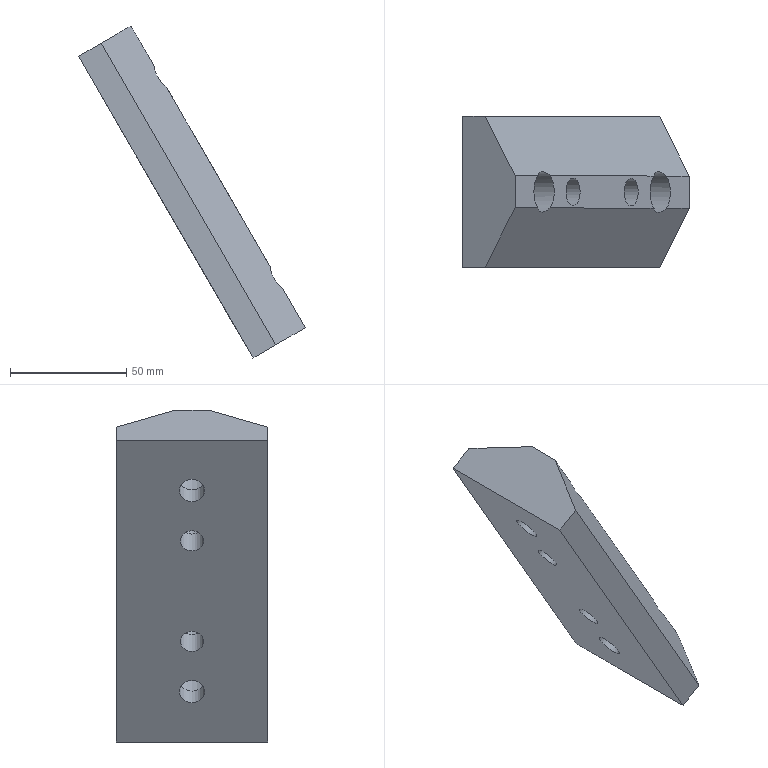Part | NX | features solid 2 | 1 solid | 22 faces | box 97.517 x 65 x 142.904 mm | volume 182430 mm3 | plane 12 | cylinder 8 | cone 2 | commonest cylinder face diameters 10 x2 11 x2 12 x2 17.5 x2
STEP:
#1=CARTESIAN_POINT('',(-987.747,-43.072,-36.314));
#2=VERTEX_POINT('',#1);
#3=CARTESIAN_POINT('',(-977.919,-43.072,-53.336));
#4=VERTEX_POINT('',#3);
#5=CARTESIAN_POINT('',(-1052.919,-43.072,76.567));
#6=DIRECTION('',(0.5,0.,-0.866));
#7=VECTOR('',#6,1000.);
#8=LINE('',#5,#7);
#9=EDGE_CURVE('',#2,#4,#8,.T.);
#10=ORIENTED_EDGE('',*,*,#9,.F.);
#11=CARTESIAN_POINT('',(-987.747,-56.928,-36.314));
#12=VERTEX_POINT('',#11);
#13=CARTESIAN_POINT('',(-990.419,-50.,-31.686));
#14=DIRECTION('',(0.866,0.,0.5));
#15=DIRECTION('',(0.5,0.,-0.866));
#16=AXIS2_PLACEMENT_3D('',#13,#14,#15);
#17=CIRCLE('',#16,8.75);
#18=EDGE_CURVE('',#12,#2,#17,.T.);
#19=ORIENTED_EDGE('',*,*,#18,.F.);
#20=CARTESIAN_POINT('',(-977.919,-56.928,-53.336));
#21=VERTEX_POINT('',#20);
#22=CARTESIAN_POINT('',(-1052.919,-56.928,76.567));
#23=DIRECTION('',(0.5,0.,-0.866));
#24=VECTOR('',#23,1000.);
#25=LINE('',#22,#24);
#26=EDGE_CURVE('',#12,#21,#25,.T.);
#27=ORIENTED_EDGE('',*,*,#26,.T.);
#28=CARTESIAN_POINT('',(-977.919,-17.5,-53.336));
#29=DIRECTION('',(0.,-1.,0.));
#30=VECTOR('',#29,1000.);
#31=LINE('',#28,#30);
#32=EDGE_CURVE('',#4,#21,#31,.T.);
#33=ORIENTED_EDGE('',*,*,#32,.F.);
#34=EDGE_LOOP('',(#10,#19,#27,#33));
#35=FACE_BOUND('',#34,.T.);
#36=CARTESIAN_POINT('',(-977.919,-17.5,-53.336));
#37=DIRECTION('',(-0.866,0.,-0.5));
#38=DIRECTION('',(0.5,0.,-0.866));
#39=AXIS2_PLACEMENT_3D('',#36,#37,#38);
#40=PLANE('',#39);
#41=ADVANCED_FACE('',(#35),#40,.F.);
#42=CARTESIAN_POINT('',(-1037.747,-43.072,50.288));
#43=VERTEX_POINT('',#42);
#44=CARTESIAN_POINT('',(-993.092,-43.072,-27.057));
#45=VERTEX_POINT('',#44);
#46=CARTESIAN_POINT('',(-1052.919,-43.072,76.567));
#47=DIRECTION('',(0.5,0.,-0.866));
#48=VECTOR('',#47,1000.);
#49=LINE('',#46,#48);
#50=EDGE_CURVE('',#43,#45,#49,.T.);
#51=ORIENTED_EDGE('',*,*,#50,.F.);
#52=CARTESIAN_POINT('',(-1037.747,-56.928,50.288));
#53=VERTEX_POINT('',#52);
#54=CARTESIAN_POINT('',(-1040.419,-50.,54.917));
#55=DIRECTION('',(0.866,0.,0.5));
#56=DIRECTION('',(0.5,0.,-0.866));
#57=AXIS2_PLACEMENT_3D('',#54,#55,#56);
#58=CIRCLE('',#57,8.75);
#59=EDGE_CURVE('',#53,#43,#58,.T.);
#60=ORIENTED_EDGE('',*,*,#59,.F.);
#61=CARTESIAN_POINT('',(-993.092,-56.928,-27.057));
#62=VERTEX_POINT('',#61);
#63=CARTESIAN_POINT('',(-1052.919,-56.928,76.567));
#64=DIRECTION('',(0.5,0.,-0.866));
#65=VECTOR('',#64,1000.);
#66=LINE('',#63,#65);
#67=EDGE_CURVE('',#53,#62,#66,.T.);
#68=ORIENTED_EDGE('',*,*,#67,.T.);
#69=CARTESIAN_POINT('',(-990.419,-50.,-31.686));
#70=DIRECTION('',(0.866,0.,0.5));
#71=DIRECTION('',(0.5,0.,-0.866));
#72=AXIS2_PLACEMENT_3D('',#69,#70,#71);
#73=CIRCLE('',#72,8.75);
#74=EDGE_CURVE('',#45,#62,#73,.T.);
#75=ORIENTED_EDGE('',*,*,#74,.F.);
#76=EDGE_LOOP('',(#51,#60,#68,#75));
#77=FACE_BOUND('',#76,.T.);
#78=CARTESIAN_POINT('',(-999.919,-50.,-15.231));
#79=VERTEX_POINT('',#78);
#80=CARTESIAN_POINT('',(-1002.919,-50.,-10.035));
#81=DIRECTION('',(0.866,0.,0.5));
#82=DIRECTION('',(0.5,0.,-0.866));
#83=AXIS2_PLACEMENT_3D('',#80,#81,#82);
#84=CIRCLE('',#83,6.);
#85=EDGE_CURVE('',#79,#79,#84,.T.);
#86=ORIENTED_EDGE('',*,*,#85,.F.);
#87=EDGE_LOOP('',(#86));
#88=FACE_BOUND('',#87,.T.);
#89=CARTESIAN_POINT('',(-1024.919,-50.,28.07));
#90=VERTEX_POINT('',#89);
#91=CARTESIAN_POINT('',(-1027.919,-50.,33.266));
#92=DIRECTION('',(0.866,0.,0.5));
#93=DIRECTION('',(0.5,0.,-0.866));
#94=AXIS2_PLACEMENT_3D('',#91,#92,#93);
#95=CIRCLE('',#94,6.);
#96=EDGE_CURVE('',#90,#90,#95,.T.);
#97=ORIENTED_EDGE('',*,*,#96,.F.);
#98=EDGE_LOOP('',(#97));
#99=FACE_BOUND('',#98,.T.);
#100=CARTESIAN_POINT('',(-977.919,-17.5,-53.336));
#101=DIRECTION('',(-0.866,0.,-0.5));
#102=DIRECTION('',(0.5,0.,-0.866));
#103=AXIS2_PLACEMENT_3D('',#100,#101,#102);
#104=PLANE('',#103);
#105=ADVANCED_FACE('',(#77,#88,#99),#104,.F.);
#106=CARTESIAN_POINT('',(-990.705,-17.5,-60.718));
#107=VERTEX_POINT('',#106);
#108=CARTESIAN_POINT('',(-977.919,-43.072,-53.336));
#109=DIRECTION('',(-0.433,0.866,-0.25));
#110=VECTOR('',#109,1000.);
#111=LINE('',#108,#110);
#112=EDGE_CURVE('',#4,#107,#111,.T.);
#113=ORIENTED_EDGE('',*,*,#112,.F.);
#114=ORIENTED_EDGE('',*,*,#32,.T.);
#115=CARTESIAN_POINT('',(-990.705,-82.5,-60.718));
#116=VERTEX_POINT('',#115);
#117=CARTESIAN_POINT('',(-990.705,-82.5,-60.718));
#118=DIRECTION('',(0.433,0.866,0.25));
#119=VECTOR('',#118,1000.);
#120=LINE('',#117,#119);
#121=EDGE_CURVE('',#116,#21,#120,.T.);
#122=ORIENTED_EDGE('',*,*,#121,.F.);
#123=CARTESIAN_POINT('',(-1000.436,-82.5,-66.336));
#124=VERTEX_POINT('',#123);
#125=CARTESIAN_POINT('',(-977.919,-82.5,-53.336));
#126=DIRECTION('',(-0.866,0.,-0.5));
#127=VECTOR('',#126,1000.);
#128=LINE('',#125,#127);
#129=EDGE_CURVE('',#116,#124,#128,.T.);
#130=ORIENTED_EDGE('',*,*,#129,.T.);
#131=CARTESIAN_POINT('',(-1000.436,-17.5,-66.336));
#132=VERTEX_POINT('',#131);
#133=CARTESIAN_POINT('',(-1000.436,-17.5,-66.336));
#134=DIRECTION('',(0.,-1.,0.));
#135=VECTOR('',#134,1000.);
#136=LINE('',#133,#135);
#137=EDGE_CURVE('',#132,#124,#136,.T.);
#138=ORIENTED_EDGE('',*,*,#137,.F.);
#139=CARTESIAN_POINT('',(-977.919,-17.5,-53.336));
#140=DIRECTION('',(-0.866,0.,-0.5));
#141=VECTOR('',#140,1000.);
#142=LINE('',#139,#141);
#143=EDGE_CURVE('',#107,#132,#142,.T.);
#144=ORIENTED_EDGE('',*,*,#143,.F.);
#145=EDGE_LOOP('',(#113,#114,#122,#130,#138,#144));
#146=FACE_BOUND('',#145,.T.);
#147=CARTESIAN_POINT('',(-977.919,-17.5,-53.336));
#148=DIRECTION('',(-0.5,0.,0.866));
#149=DIRECTION('',(0.,1.,0.));
#150=AXIS2_PLACEMENT_3D('',#147,#148,#149);
#151=PLANE('',#150);
#152=ADVANCED_FACE('',(#146),#151,.F.);
#153=CARTESIAN_POINT('',(-1065.705,-82.5,69.185));
#154=VERTEX_POINT('',#153);
#155=CARTESIAN_POINT('',(-1065.705,-82.5,69.185));
#156=DIRECTION('',(0.5,0.,-0.866));
#157=VECTOR('',#156,1000.);
#158=LINE('',#155,#157);
#159=EDGE_CURVE('',#154,#116,#158,.T.);
#160=ORIENTED_EDGE('',*,*,#159,.F.);
#161=CARTESIAN_POINT('',(-1075.436,-82.5,63.567));
#162=VERTEX_POINT('',#161);
#163=CARTESIAN_POINT('',(-1052.919,-82.5,76.567));
#164=DIRECTION('',(-0.866,0.,-0.5));
#165=VECTOR('',#164,1000.);
#166=LINE('',#163,#165);
#167=EDGE_CURVE('',#154,#162,#166,.T.);
#168=ORIENTED_EDGE('',*,*,#167,.T.);
#169=CARTESIAN_POINT('',(-1000.436,-82.5,-66.336));
#170=DIRECTION('',(-0.5,0.,0.866));
#171=VECTOR('',#170,1000.);
#172=LINE('',#169,#171);
#173=EDGE_CURVE('',#124,#162,#172,.T.);
#174=ORIENTED_EDGE('',*,*,#173,.F.);
#175=ORIENTED_EDGE('',*,*,#129,.F.);
#176=EDGE_LOOP('',(#160,#168,#174,#175));
#177=FACE_BOUND('',#176,.T.);
#178=CARTESIAN_POINT('',(-977.919,-82.5,-53.336));
#179=DIRECTION('',(0.,1.,0.));
#180=DIRECTION('',(0.5,0.,-0.866));
#181=AXIS2_PLACEMENT_3D('',#178,#179,#180);
#182=PLANE('',#181);
#183=ADVANCED_FACE('',(#177),#182,.F.);
#184=CARTESIAN_POINT('',(-1052.919,-43.072,76.567));
#185=VERTEX_POINT('',#184);
#186=CARTESIAN_POINT('',(-1065.705,-17.5,69.185));
#187=VERTEX_POINT('',#186);
#188=CARTESIAN_POINT('',(-1052.919,-43.072,76.567));
#189=DIRECTION('',(-0.433,0.866,-0.25));
#190=VECTOR('',#189,1000.);
#191=LINE('',#188,#190);
#192=EDGE_CURVE('',#185,#187,#191,.T.);
#193=ORIENTED_EDGE('',*,*,#192,.T.);
#194=CARTESIAN_POINT('',(-1075.436,-17.5,63.567));
#195=VERTEX_POINT('',#194);
#196=CARTESIAN_POINT('',(-1052.919,-17.5,76.567));
#197=DIRECTION('',(-0.866,0.,-0.5));
#198=VECTOR('',#197,1000.);
#199=LINE('',#196,#198);
#200=EDGE_CURVE('',#187,#195,#199,.T.);
#201=ORIENTED_EDGE('',*,*,#200,.T.);
#202=CARTESIAN_POINT('',(-1075.436,-82.5,63.567));
#203=DIRECTION('',(0.,1.,0.));
#204=VECTOR('',#203,1000.);
#205=LINE('',#202,#204);
#206=EDGE_CURVE('',#162,#195,#205,.T.);
#207=ORIENTED_EDGE('',*,*,#206,.F.);
#208=ORIENTED_EDGE('',*,*,#167,.F.);
#209=CARTESIAN_POINT('',(-1052.919,-56.928,76.567));
#210=VERTEX_POINT('',#209);
#211=CARTESIAN_POINT('',(-1065.705,-82.5,69.185));
#212=DIRECTION('',(0.433,0.866,0.25));
#213=VECTOR('',#212,1000.);
#214=LINE('',#211,#213);
#215=EDGE_CURVE('',#154,#210,#214,.T.);
#216=ORIENTED_EDGE('',*,*,#215,.T.);
#217=CARTESIAN_POINT('',(-1052.919,-82.5,76.567));
#218=DIRECTION('',(0.,1.,0.));
#219=VECTOR('',#218,1000.);
#220=LINE('',#217,#219);
#221=EDGE_CURVE('',#210,#185,#220,.T.);
#222=ORIENTED_EDGE('',*,*,#221,.T.);
#223=EDGE_LOOP('',(#193,#201,#207,#208,#216,#222));
#224=FACE_BOUND('',#223,.T.);
#225=CARTESIAN_POINT('',(-1052.919,-82.5,76.567));
#226=DIRECTION('',(0.5,0.,-0.866));
#227=DIRECTION('',(0.866,0.,0.5));
#228=AXIS2_PLACEMENT_3D('',#225,#226,#227);
#229=PLANE('',#228);
#230=ADVANCED_FACE('',(#224),#229,.F.);
#231=CARTESIAN_POINT('',(-1065.705,-17.5,69.185));
#232=DIRECTION('',(0.5,0.,-0.866));
#233=VECTOR('',#232,1000.);
#234=LINE('',#231,#233);
#235=EDGE_CURVE('',#187,#107,#234,.T.);
#236=ORIENTED_EDGE('',*,*,#235,.T.);
#237=ORIENTED_EDGE('',*,*,#143,.T.);
#238=CARTESIAN_POINT('',(-1075.436,-17.5,63.567));
#239=DIRECTION('',(0.5,0.,-0.866));
#240=VECTOR('',#239,1000.);
#241=LINE('',#238,#240);
#242=EDGE_CURVE('',#195,#132,#241,.T.);
#243=ORIENTED_EDGE('',*,*,#242,.F.);
#244=ORIENTED_EDGE('',*,*,#200,.F.);
#245=EDGE_LOOP('',(#236,#237,#243,#244));
#246=FACE_BOUND('',#245,.T.);
#247=CARTESIAN_POINT('',(-1052.919,-17.5,76.567));
#248=DIRECTION('',(0.,-1.,0.));
#249=DIRECTION('',(-0.5,0.,0.866));
#250=AXIS2_PLACEMENT_3D('',#247,#248,#249);
#251=PLANE('',#250);
#252=ADVANCED_FACE('',(#246),#251,.F.);
#253=CARTESIAN_POINT('',(-1043.092,-43.072,59.545));
#254=VERTEX_POINT('',#253);
#255=CARTESIAN_POINT('',(-1052.919,-43.072,76.567));
#256=DIRECTION('',(0.5,0.,-0.866));
#257=VECTOR('',#256,1000.);
#258=LINE('',#255,#257);
#259=EDGE_CURVE('',#185,#254,#258,.T.);
#260=ORIENTED_EDGE('',*,*,#259,.F.);
#261=ORIENTED_EDGE('',*,*,#221,.F.);
#262=CARTESIAN_POINT('',(-1043.092,-56.928,59.545));
#263=VERTEX_POINT('',#262);
#264=CARTESIAN_POINT('',(-1052.919,-56.928,76.567));
#265=DIRECTION('',(0.5,0.,-0.866));
#266=VECTOR('',#265,1000.);
#267=LINE('',#264,#266);
#268=EDGE_CURVE('',#210,#263,#267,.T.);
#269=ORIENTED_EDGE('',*,*,#268,.T.);
#270=CARTESIAN_POINT('',(-1040.419,-50.,54.917));
#271=DIRECTION('',(0.866,0.,0.5));
#272=DIRECTION('',(0.5,0.,-0.866));
#273=AXIS2_PLACEMENT_3D('',#270,#271,#272);
#274=CIRCLE('',#273,8.75);
#275=EDGE_CURVE('',#254,#263,#274,.T.);
#276=ORIENTED_EDGE('',*,*,#275,.F.);
#277=EDGE_LOOP('',(#260,#261,#269,#276));
#278=FACE_BOUND('',#277,.T.);
#279=CARTESIAN_POINT('',(-977.919,-17.5,-53.336));
#280=DIRECTION('',(-0.866,0.,-0.5));
#281=DIRECTION('',(0.5,0.,-0.866));
#282=AXIS2_PLACEMENT_3D('',#279,#280,#281);
#283=PLANE('',#282);
#284=ADVANCED_FACE('',(#278),#283,.F.);
#285=CARTESIAN_POINT('',(-1052.936,-50.,24.596));
#286=VERTEX_POINT('',#285);
#287=CARTESIAN_POINT('',(-1050.436,-50.,20.266));
#288=DIRECTION('',(-0.866,0.,-0.5));
#289=DIRECTION('',(-0.5,0.,0.866));
#290=AXIS2_PLACEMENT_3D('',#287,#288,#289);
#291=CIRCLE('',#290,5.);
#292=EDGE_CURVE('',#286,#286,#291,.T.);
#293=ORIENTED_EDGE('',*,*,#292,.F.);
#294=EDGE_LOOP('',(#293));
#295=FACE_BOUND('',#294,.T.);
#296=CARTESIAN_POINT('',(-1027.936,-50.,-18.705));
#297=VERTEX_POINT('',#296);
#298=CARTESIAN_POINT('',(-1025.436,-50.,-23.035));
#299=DIRECTION('',(-0.866,0.,-0.5));
#300=DIRECTION('',(-0.5,0.,0.866));
#301=AXIS2_PLACEMENT_3D('',#298,#299,#300);
#302=CIRCLE('',#301,5.);
#303=EDGE_CURVE('',#297,#297,#302,.T.);
#304=ORIENTED_EDGE('',*,*,#303,.F.);
#305=EDGE_LOOP('',(#304));
#306=FACE_BOUND('',#305,.T.);
#307=CARTESIAN_POINT('',(-1065.686,-50.,46.68));
#308=VERTEX_POINT('',#307);
#309=CARTESIAN_POINT('',(-1062.936,-50.,41.917));
#310=DIRECTION('',(-0.866,0.,-0.5));
#311=DIRECTION('',(-0.5,0.,0.866));
#312=AXIS2_PLACEMENT_3D('',#309,#310,#311);
#313=CIRCLE('',#312,5.5);
#314=EDGE_CURVE('',#308,#308,#313,.F.);
#315=ORIENTED_EDGE('',*,*,#314,.T.);
#316=EDGE_LOOP('',(#315));
#317=FACE_BOUND('',#316,.T.);
#318=CARTESIAN_POINT('',(-1015.686,-50.,-39.923));
#319=VERTEX_POINT('',#318);
#320=CARTESIAN_POINT('',(-1012.936,-50.,-44.686));
#321=DIRECTION('',(-0.866,0.,-0.5));
#322=DIRECTION('',(-0.5,0.,0.866));
#323=AXIS2_PLACEMENT_3D('',#320,#321,#322);
#324=CIRCLE('',#323,5.5);
#325=EDGE_CURVE('',#319,#319,#324,.F.);
#326=ORIENTED_EDGE('',*,*,#325,.T.);
#327=EDGE_LOOP('',(#326));
#328=FACE_BOUND('',#327,.T.);
#329=ORIENTED_EDGE('',*,*,#137,.T.);
#330=ORIENTED_EDGE('',*,*,#173,.T.);
#331=ORIENTED_EDGE('',*,*,#206,.T.);
#332=ORIENTED_EDGE('',*,*,#242,.T.);
#333=EDGE_LOOP('',(#329,#330,#331,#332));
#334=FACE_BOUND('',#333,.T.);
#335=CARTESIAN_POINT('',(-1000.436,-17.5,-66.336));
#336=DIRECTION('',(-0.866,0.,-0.5));
#337=DIRECTION('',(0.5,0.,-0.866));
#338=AXIS2_PLACEMENT_3D('',#335,#336,#337);
#339=PLANE('',#338);
#340=ADVANCED_FACE('',(#295,#306,#317,#328,#334),#339,.T.);
#341=ORIENTED_EDGE('',*,*,#325,.F.);
#342=EDGE_LOOP('',(#341));
#343=FACE_BOUND('',#342,.T.);
#344=CARTESIAN_POINT('',(-1001.526,-50.,-44.449));
#345=VERTEX_POINT('',#344);
#346=CARTESIAN_POINT('',(-1004.276,-50.,-39.686));
#347=DIRECTION('',(0.866,0.,0.5));
#348=DIRECTION('',(0.5,0.,-0.866));
#349=AXIS2_PLACEMENT_3D('',#346,#347,#348);
#350=CIRCLE('',#349,5.5);
#351=EDGE_CURVE('',#345,#345,#350,.T.);
#352=ORIENTED_EDGE('',*,*,#351,.T.);
#353=EDGE_LOOP('',(#352));
#354=FACE_BOUND('',#353,.T.);
#355=CARTESIAN_POINT('',(-1012.936,-50.,-44.686));
#356=DIRECTION('',(-0.866,0.,-0.5));
#357=DIRECTION('',(0.5,0.,-0.866));
#358=AXIS2_PLACEMENT_3D('',#355,#356,#357);
#359=CYLINDRICAL_SURFACE('',#358,5.5);
#360=ADVANCED_FACE('',(#343,#354),#359,.F.);
#361=ORIENTED_EDGE('',*,*,#351,.F.);
#362=EDGE_LOOP('',(#361));
#363=FACE_BOUND('',#362,.T.);
#364=CARTESIAN_POINT('',(-999.901,-50.,-47.264));
#365=VERTEX_POINT('',#364);
#366=CARTESIAN_POINT('',(-1004.276,-50.,-39.686));
#367=DIRECTION('',(0.866,0.,0.5));
#368=DIRECTION('',(0.5,0.,-0.866));
#369=AXIS2_PLACEMENT_3D('',#366,#367,#368);
#370=CIRCLE('',#369,8.75);
#371=EDGE_CURVE('',#365,#365,#370,.T.);
#372=ORIENTED_EDGE('',*,*,#371,.T.);
#373=EDGE_LOOP('',(#372));
#374=FACE_BOUND('',#373,.T.);
#375=CARTESIAN_POINT('',(-1004.276,-50.,-39.686));
#376=DIRECTION('',(-0.866,0.,-0.5));
#377=DIRECTION('',(0.5,0.,-0.866));
#378=AXIS2_PLACEMENT_3D('',#375,#376,#377);
#379=PLANE('',#378);
#380=ADVANCED_FACE('',(#363,#374),#379,.F.);
#381=CARTESIAN_POINT('',(-986.955,-50.,-29.686));
#382=DIRECTION('',(-0.75,-0.5,-0.433));
#383=DIRECTION('',(-0.433,0.866,-0.25));
#384=AXIS2_PLACEMENT_3D('',#381,#382,#383);
#385=ELLIPSE('',#384,10.104,8.75);
#386=EDGE_CURVE('',#2,#45,#385,.F.);
#387=ORIENTED_EDGE('',*,*,#386,.T.);
#388=ORIENTED_EDGE('',*,*,#74,.T.);
#389=CARTESIAN_POINT('',(-986.955,-50.,-29.686));
#390=DIRECTION('',(-0.75,0.5,-0.433));
#391=DIRECTION('',(-0.433,-0.866,-0.25));
#392=AXIS2_PLACEMENT_3D('',#389,#390,#391);
#393=ELLIPSE('',#392,10.104,8.75);
#394=EDGE_CURVE('',#62,#12,#393,.F.);
#395=ORIENTED_EDGE('',*,*,#394,.T.);
#396=ORIENTED_EDGE('',*,*,#18,.T.);
#397=EDGE_LOOP('',(#387,#388,#395,#396));
#398=FACE_BOUND('',#397,.T.);
#399=ORIENTED_EDGE('',*,*,#371,.F.);
#400=EDGE_LOOP('',(#399));
#401=FACE_BOUND('',#400,.T.);
#402=CARTESIAN_POINT('',(-990.419,-50.,-31.686));
#403=DIRECTION('',(-0.866,0.,-0.5));
#404=DIRECTION('',(0.5,0.,-0.866));
#405=AXIS2_PLACEMENT_3D('',#402,#403,#404);
#406=CYLINDRICAL_SURFACE('',#405,8.75);
#407=ADVANCED_FACE('',(#398,#401),#406,.F.);
#408=ORIENTED_EDGE('',*,*,#314,.F.);
#409=EDGE_LOOP('',(#408));
#410=FACE_BOUND('',#409,.T.);
#411=CARTESIAN_POINT('',(-1051.526,-50.,42.154));
#412=VERTEX_POINT('',#411);
#413=CARTESIAN_POINT('',(-1054.276,-50.,46.917));
#414=DIRECTION('',(0.866,0.,0.5));
#415=DIRECTION('',(0.5,0.,-0.866));
#416=AXIS2_PLACEMENT_3D('',#413,#414,#415);
#417=CIRCLE('',#416,5.5);
#418=EDGE_CURVE('',#412,#412,#417,.T.);
#419=ORIENTED_EDGE('',*,*,#418,.T.);
#420=EDGE_LOOP('',(#419));
#421=FACE_BOUND('',#420,.T.);
#422=CARTESIAN_POINT('',(-1062.936,-50.,41.917));
#423=DIRECTION('',(-0.866,0.,-0.5));
#424=DIRECTION('',(0.5,0.,-0.866));
#425=AXIS2_PLACEMENT_3D('',#422,#423,#424);
#426=CYLINDRICAL_SURFACE('',#425,5.5);
#427=ADVANCED_FACE('',(#410,#421),#426,.F.);
#428=ORIENTED_EDGE('',*,*,#418,.F.);
#429=EDGE_LOOP('',(#428));
#430=FACE_BOUND('',#429,.T.);
#431=CARTESIAN_POINT('',(-1049.901,-50.,39.339));
#432=VERTEX_POINT('',#431);
#433=CARTESIAN_POINT('',(-1054.276,-50.,46.917));
#434=DIRECTION('',(0.866,0.,0.5));
#435=DIRECTION('',(0.5,0.,-0.866));
#436=AXIS2_PLACEMENT_3D('',#433,#434,#435);
#437=CIRCLE('',#436,8.75);
#438=EDGE_CURVE('',#432,#432,#437,.T.);
#439=ORIENTED_EDGE('',*,*,#438,.T.);
#440=EDGE_LOOP('',(#439));
#441=FACE_BOUND('',#440,.T.);
#442=CARTESIAN_POINT('',(-1054.276,-50.,46.917));
#443=DIRECTION('',(-0.866,0.,-0.5));
#444=DIRECTION('',(0.5,0.,-0.866));
#445=AXIS2_PLACEMENT_3D('',#442,#443,#444);
#446=PLANE('',#445);
#447=ADVANCED_FACE('',(#430,#441),#446,.F.);
#448=CARTESIAN_POINT('',(-1036.955,-50.,56.917));
#449=DIRECTION('',(-0.75,-0.5,-0.433));
#450=DIRECTION('',(-0.433,0.866,-0.25));
#451=AXIS2_PLACEMENT_3D('',#448,#449,#450);
#452=ELLIPSE('',#451,10.104,8.75);
#453=EDGE_CURVE('',#43,#254,#452,.F.);
#454=ORIENTED_EDGE('',*,*,#453,.T.);
#455=ORIENTED_EDGE('',*,*,#275,.T.);
#456=CARTESIAN_POINT('',(-1036.955,-50.,56.917));
#457=DIRECTION('',(-0.75,0.5,-0.433));
#458=DIRECTION('',(-0.433,-0.866,-0.25));
#459=AXIS2_PLACEMENT_3D('',#456,#457,#458);
#460=ELLIPSE('',#459,10.104,8.75);
#461=EDGE_CURVE('',#263,#53,#460,.F.);
#462=ORIENTED_EDGE('',*,*,#461,.T.);
#463=ORIENTED_EDGE('',*,*,#59,.T.);
#464=EDGE_LOOP('',(#454,#455,#462,#463));
#465=FACE_BOUND('',#464,.T.);
#466=ORIENTED_EDGE('',*,*,#438,.F.);
#467=EDGE_LOOP('',(#466));
#468=FACE_BOUND('',#467,.T.);
#469=CARTESIAN_POINT('',(-1040.419,-50.,54.917));
#470=DIRECTION('',(-0.866,0.,-0.5));
#471=DIRECTION('',(0.5,0.,-0.866));
#472=AXIS2_PLACEMENT_3D('',#469,#470,#471);
#473=CYLINDRICAL_SURFACE('',#472,8.75);
#474=ADVANCED_FACE('',(#465,#468),#473,.F.);
#475=CARTESIAN_POINT('',(-1015.446,-50.,-11.494));
#476=VERTEX_POINT('',#475);
#477=CARTESIAN_POINT('',(-1012.946,-50.,-15.824));
#478=DIRECTION('',(-0.866,0.,-0.5));
#479=DIRECTION('',(-0.5,0.,0.866));
#480=AXIS2_PLACEMENT_3D('',#477,#478,#479);
#481=CIRCLE('',#480,5.);
#482=EDGE_CURVE('',#476,#476,#481,.F.);
#483=ORIENTED_EDGE('',*,*,#482,.F.);
#484=EDGE_LOOP('',(#483));
#485=FACE_BOUND('',#484,.T.);
#486=CARTESIAN_POINT('',(-1009.446,-50.,-20.731));
#487=VERTEX_POINT('',#486);
#488=CARTESIAN_POINT('',(-1012.446,-50.,-15.535));
#489=DIRECTION('',(0.866,0.,0.5));
#490=DIRECTION('',(0.5,0.,-0.866));
#491=AXIS2_PLACEMENT_3D('',#488,#489,#490);
#492=CIRCLE('',#491,6.);
#493=EDGE_CURVE('',#487,#487,#492,.T.);
#494=ORIENTED_EDGE('',*,*,#493,.T.);
#495=EDGE_LOOP('',(#494));
#496=FACE_BOUND('',#495,.T.);
#497=CARTESIAN_POINT('',(-1012.446,-50.,-15.535));
#498=DIRECTION('',(0.866,0.,0.5));
#499=DIRECTION('',(-0.5,0.,0.866));
#500=AXIS2_PLACEMENT_3D('',#497,#498,#499);
#501=CONICAL_SURFACE('',#500,6.,1.047);
#502=ADVANCED_FACE('',(#485,#496),#501,.F.);
#503=ORIENTED_EDGE('',*,*,#493,.F.);
#504=EDGE_LOOP('',(#503));
#505=FACE_BOUND('',#504,.T.);
#506=ORIENTED_EDGE('',*,*,#85,.T.);
#507=EDGE_LOOP('',(#506));
#508=FACE_BOUND('',#507,.T.);
#509=CARTESIAN_POINT('',(-1002.919,-50.,-10.035));
#510=DIRECTION('',(-0.866,0.,-0.5));
#511=DIRECTION('',(0.5,0.,-0.866));
#512=AXIS2_PLACEMENT_3D('',#509,#510,#511);
#513=CYLINDRICAL_SURFACE('',#512,6.);
#514=ADVANCED_FACE('',(#505,#508),#513,.F.);
#515=CARTESIAN_POINT('',(-1040.446,-50.,31.808));
#516=VERTEX_POINT('',#515);
#517=CARTESIAN_POINT('',(-1037.946,-50.,27.477));
#518=DIRECTION('',(-0.866,0.,-0.5));
#519=DIRECTION('',(-0.5,0.,0.866));
#520=AXIS2_PLACEMENT_3D('',#517,#518,#519);
#521=CIRCLE('',#520,5.);
#522=EDGE_CURVE('',#516,#516,#521,.F.);
#523=ORIENTED_EDGE('',*,*,#522,.F.);
#524=EDGE_LOOP('',(#523));
#525=FACE_BOUND('',#524,.T.);
#526=CARTESIAN_POINT('',(-1034.446,-50.,22.57));
#527=VERTEX_POINT('',#526);
#528=CARTESIAN_POINT('',(-1037.446,-50.,27.766));
#529=DIRECTION('',(0.866,0.,0.5));
#530=DIRECTION('',(0.5,0.,-0.866));
#531=AXIS2_PLACEMENT_3D('',#528,#529,#530);
#532=CIRCLE('',#531,6.);
#533=EDGE_CURVE('',#527,#527,#532,.T.);
#534=ORIENTED_EDGE('',*,*,#533,.T.);
#535=EDGE_LOOP('',(#534));
#536=FACE_BOUND('',#535,.T.);
#537=CARTESIAN_POINT('',(-1037.446,-50.,27.766));
#538=DIRECTION('',(0.866,0.,0.5));
#539=DIRECTION('',(-0.5,0.,0.866));
#540=AXIS2_PLACEMENT_3D('',#537,#538,#539);
#541=CONICAL_SURFACE('',#540,6.,1.047);
#542=ADVANCED_FACE('',(#525,#536),#541,.F.);
#543=ORIENTED_EDGE('',*,*,#533,.F.);
#544=EDGE_LOOP('',(#543));
#545=FACE_BOUND('',#544,.T.);
#546=ORIENTED_EDGE('',*,*,#96,.T.);
#547=EDGE_LOOP('',(#546));
#548=FACE_BOUND('',#547,.T.);
#549=CARTESIAN_POINT('',(-1027.919,-50.,33.266));
#550=DIRECTION('',(-0.866,0.,-0.5));
#551=DIRECTION('',(0.5,0.,-0.866));
#552=AXIS2_PLACEMENT_3D('',#549,#550,#551);
#553=CYLINDRICAL_SURFACE('',#552,6.);
#554=ADVANCED_FACE('',(#545,#548),#553,.F.);
#555=ORIENTED_EDGE('',*,*,#303,.T.);
#556=EDGE_LOOP('',(#555));
#557=FACE_BOUND('',#556,.T.);
#558=ORIENTED_EDGE('',*,*,#482,.T.);
#559=EDGE_LOOP('',(#558));
#560=FACE_BOUND('',#559,.T.);
#561=CARTESIAN_POINT('',(-1025.436,-50.,-23.035));
#562=DIRECTION('',(0.866,0.,0.5));
#563=DIRECTION('',(-0.5,0.,0.866));
#564=AXIS2_PLACEMENT_3D('',#561,#562,#563);
#565=CYLINDRICAL_SURFACE('',#564,5.);
#566=ADVANCED_FACE('',(#557,#560),#565,.F.);
#567=ORIENTED_EDGE('',*,*,#292,.T.);
#568=EDGE_LOOP('',(#567));
#569=FACE_BOUND('',#568,.T.);
#570=ORIENTED_EDGE('',*,*,#522,.T.);
#571=EDGE_LOOP('',(#570));
#572=FACE_BOUND('',#571,.T.);
#573=CARTESIAN_POINT('',(-1050.436,-50.,20.266));
#574=DIRECTION('',(0.866,0.,0.5));
#575=DIRECTION('',(-0.5,0.,0.866));
#576=AXIS2_PLACEMENT_3D('',#573,#574,#575);
#577=CYLINDRICAL_SURFACE('',#576,5.);
#578=ADVANCED_FACE('',(#569,#572),#577,.F.);
#579=ORIENTED_EDGE('',*,*,#67,.F.);
#580=ORIENTED_EDGE('',*,*,#461,.F.);
#581=ORIENTED_EDGE('',*,*,#268,.F.);
#582=ORIENTED_EDGE('',*,*,#215,.F.);
#583=ORIENTED_EDGE('',*,*,#159,.T.);
#584=ORIENTED_EDGE('',*,*,#121,.T.);
#585=ORIENTED_EDGE('',*,*,#26,.F.);
#586=ORIENTED_EDGE('',*,*,#394,.F.);
#587=EDGE_LOOP('',(#579,#580,#581,#582,#583,#584,#585,#586));
#588=FACE_BOUND('',#587,.T.);
#589=CARTESIAN_POINT('',(-1065.705,-82.5,69.185));
#590=DIRECTION('',(0.75,-0.5,0.433));
#591=DIRECTION('',(-0.433,-0.866,-0.25));
#592=AXIS2_PLACEMENT_3D('',#589,#590,#591);
#593=PLANE('',#592);
#594=ADVANCED_FACE('',(#588),#593,.T.);
#595=ORIENTED_EDGE('',*,*,#9,.T.);
#596=ORIENTED_EDGE('',*,*,#112,.T.);
#597=ORIENTED_EDGE('',*,*,#235,.F.);
#598=ORIENTED_EDGE('',*,*,#192,.F.);
#599=ORIENTED_EDGE('',*,*,#259,.T.);
#600=ORIENTED_EDGE('',*,*,#453,.F.);
#601=ORIENTED_EDGE('',*,*,#50,.T.);
#602=ORIENTED_EDGE('',*,*,#386,.F.);
#603=EDGE_LOOP('',(#595,#596,#597,#598,#599,#600,#601,#602));
#604=FACE_BOUND('',#603,.T.);
#605=CARTESIAN_POINT('',(-1052.919,-43.072,76.567));
#606=DIRECTION('',(0.75,0.5,0.433));
#607=DIRECTION('',(0.433,-0.866,0.25));
#608=AXIS2_PLACEMENT_3D('',#605,#606,#607);
#609=PLANE('',#608);
#610=ADVANCED_FACE('',(#604),#609,.T.);
#611=CLOSED_SHELL('',(#41,#105,#152,#183,#230,#252,#284,#340,#360,#380,#407,#427,#447,#474,#502,#514,#542,#554,#566,#578,#594,#610));
#612=MANIFOLD_SOLID_BREP('',#611);
#613=(LENGTH_UNIT()NAMED_UNIT(*)SI_UNIT(.MILLI.,.METRE.));
#614=UNCERTAINTY_MEASURE_WITH_UNIT(LENGTH_MEASURE(0.00001),#613,'','');
#615=(NAMED_UNIT(*)PLANE_ANGLE_UNIT()SI_UNIT($,.RADIAN.));
#616=(NAMED_UNIT(*)SI_UNIT($,.STERADIAN.)SOLID_ANGLE_UNIT());
#617=(GEOMETRIC_REPRESENTATION_CONTEXT(3)GLOBAL_UNCERTAINTY_ASSIGNED_CONTEXT((#614))GLOBAL_UNIT_ASSIGNED_CONTEXT((#613,#615,#616))REPRESENTATION_CONTEXT('',''));
#618=ADVANCED_BREP_SHAPE_REPRESENTATION('',(#612),#617);